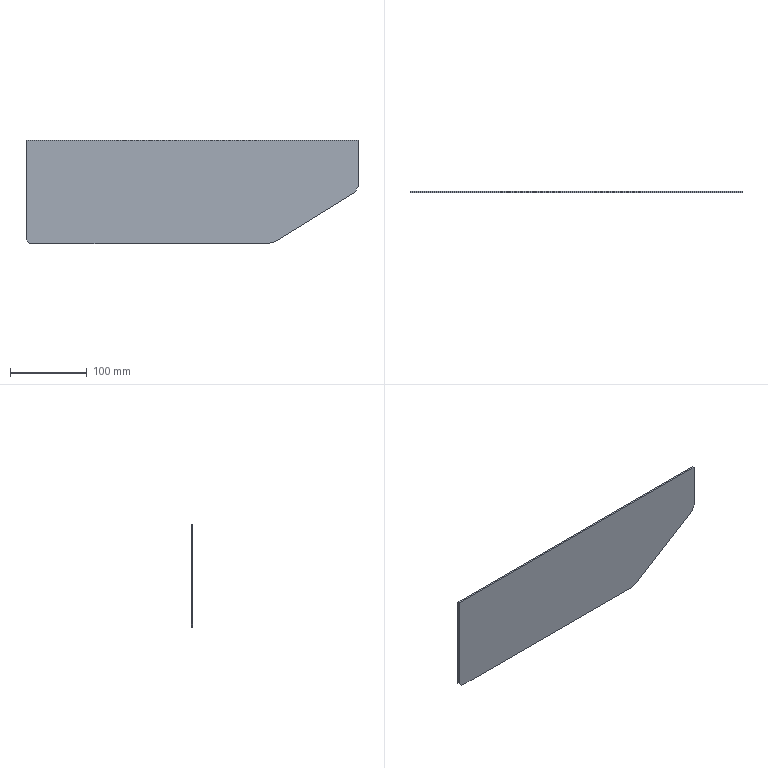Part | SolidWorks | features Chamfer 2, FlatPattern 1, SMBaseFlange 1, SheetMetal 1 | 1 solid | 10 faces | box 431.35 x 2.3 x 134 mm | volume 124034 mm3 | plane 10
STEP:
#1=CARTESIAN_POINT('',(0.,0.,-129.));
#2=VERTEX_POINT('',#1);
#3=CARTESIAN_POINT('',(0.,0.,0.));
#4=VERTEX_POINT('',#3);
#5=CARTESIAN_POINT('',(0.,0.,-134.));
#6=DIRECTION('',(0.,0.,1.));
#7=VECTOR('',#6,1000.);
#8=LINE('',#5,#7);
#9=EDGE_CURVE('',#2,#4,#8,.T.);
#10=ORIENTED_EDGE('',*,*,#9,.F.);
#11=CARTESIAN_POINT('',(0.,-2.3,-129.));
#12=VERTEX_POINT('',#11);
#13=CARTESIAN_POINT('',(0.,-2.3,-129.));
#14=DIRECTION('',(0.,-1.,0.));
#15=VECTOR('',#14,1000.);
#16=LINE('',#13,#15);
#17=EDGE_CURVE('',#2,#12,#16,.T.);
#18=ORIENTED_EDGE('',*,*,#17,.T.);
#19=CARTESIAN_POINT('',(0.,-2.3,0.));
#20=VERTEX_POINT('',#19);
#21=CARTESIAN_POINT('',(0.,-2.3,-134.));
#22=DIRECTION('',(0.,0.,1.));
#23=VECTOR('',#22,1000.);
#24=LINE('',#21,#23);
#25=EDGE_CURVE('',#12,#20,#24,.T.);
#26=ORIENTED_EDGE('',*,*,#25,.T.);
#27=CARTESIAN_POINT('',(0.,-2.3,0.));
#28=DIRECTION('',(0.,1.,0.));
#29=VECTOR('',#28,1000.);
#30=LINE('',#27,#29);
#31=EDGE_CURVE('',#20,#4,#30,.T.);
#32=ORIENTED_EDGE('',*,*,#31,.T.);
#33=EDGE_LOOP('',(#10,#18,#26,#32));
#34=FACE_OUTER_BOUND('',#33,.T.);
#35=CARTESIAN_POINT('',(0.,-2.3,-134.));
#36=DIRECTION('',(-1.,0.,0.));
#37=DIRECTION('',(0.,0.,1.));
#38=AXIS2_PLACEMENT_3D('',#35,#36,#37);
#39=PLANE('',#38);
#40=ADVANCED_FACE('',(#34),#39,.T.);
#41=CARTESIAN_POINT('',(314.95,-2.3,-134.));
#42=VERTEX_POINT('',#41);
#43=CARTESIAN_POINT('',(5.,-2.3,-134.));
#44=VERTEX_POINT('',#43);
#45=CARTESIAN_POINT('',(319.95,-2.3,-134.));
#46=DIRECTION('',(-1.,0.,0.));
#47=VECTOR('',#46,1000.);
#48=LINE('',#45,#47);
#49=EDGE_CURVE('',#42,#44,#48,.T.);
#50=ORIENTED_EDGE('',*,*,#49,.T.);
#51=CARTESIAN_POINT('',(5.,0.,-134.));
#52=VERTEX_POINT('',#51);
#53=CARTESIAN_POINT('',(5.,-2.3,-134.));
#54=DIRECTION('',(0.,1.,0.));
#55=VECTOR('',#54,1000.);
#56=LINE('',#53,#55);
#57=EDGE_CURVE('',#44,#52,#56,.T.);
#58=ORIENTED_EDGE('',*,*,#57,.T.);
#59=CARTESIAN_POINT('',(314.95,0.,-134.));
#60=VERTEX_POINT('',#59);
#61=CARTESIAN_POINT('',(319.95,0.,-134.));
#62=DIRECTION('',(-1.,0.,0.));
#63=VECTOR('',#62,1000.);
#64=LINE('',#61,#63);
#65=EDGE_CURVE('',#60,#52,#64,.T.);
#66=ORIENTED_EDGE('',*,*,#65,.F.);
#67=CARTESIAN_POINT('',(314.95,-2.3,-134.));
#68=DIRECTION('',(0.,-1.,0.));
#69=VECTOR('',#68,1000.);
#70=LINE('',#67,#69);
#71=EDGE_CURVE('',#60,#42,#70,.T.);
#72=ORIENTED_EDGE('',*,*,#71,.T.);
#73=EDGE_LOOP('',(#50,#58,#66,#72));
#74=FACE_OUTER_BOUND('',#73,.T.);
#75=CARTESIAN_POINT('',(319.95,-2.3,-134.));
#76=DIRECTION('',(0.,0.,-1.));
#77=DIRECTION('',(-1.,0.,0.));
#78=AXIS2_PLACEMENT_3D('',#75,#76,#77);
#79=PLANE('',#78);
#80=ADVANCED_FACE('',(#74),#79,.T.);
#81=CARTESIAN_POINT('',(427.099,0.,-67.633));
#82=VERTEX_POINT('',#81);
#83=CARTESIAN_POINT('',(324.201,0.,-131.367));
#84=VERTEX_POINT('',#83);
#85=CARTESIAN_POINT('',(431.35,0.,-65.));
#86=DIRECTION('',(-0.8501,0.,-0.5266));
#87=VECTOR('',#86,1000.);
#88=LINE('',#85,#87);
#89=EDGE_CURVE('',#82,#84,#88,.T.);
#90=ORIENTED_EDGE('',*,*,#89,.F.);
#91=CARTESIAN_POINT('',(427.099,-2.3,-67.633));
#92=VERTEX_POINT('',#91);
#93=CARTESIAN_POINT('',(427.099,-2.3,-67.633));
#94=DIRECTION('',(0.,-1.,0.));
#95=VECTOR('',#94,1000.);
#96=LINE('',#93,#95);
#97=EDGE_CURVE('',#82,#92,#96,.T.);
#98=ORIENTED_EDGE('',*,*,#97,.T.);
#99=CARTESIAN_POINT('',(324.201,-2.3,-131.367));
#100=VERTEX_POINT('',#99);
#101=CARTESIAN_POINT('',(431.35,-2.3,-65.));
#102=DIRECTION('',(-0.8501,0.,-0.5266));
#103=VECTOR('',#102,1000.);
#104=LINE('',#101,#103);
#105=EDGE_CURVE('',#92,#100,#104,.T.);
#106=ORIENTED_EDGE('',*,*,#105,.T.);
#107=CARTESIAN_POINT('',(324.201,-2.3,-131.367));
#108=DIRECTION('',(0.,1.,0.));
#109=VECTOR('',#108,1000.);
#110=LINE('',#107,#109);
#111=EDGE_CURVE('',#100,#84,#110,.T.);
#112=ORIENTED_EDGE('',*,*,#111,.T.);
#113=EDGE_LOOP('',(#90,#98,#106,#112));
#114=FACE_OUTER_BOUND('',#113,.T.);
#115=CARTESIAN_POINT('',(431.35,-2.3,-65.));
#116=DIRECTION('',(0.5266,0.,-0.8501));
#117=DIRECTION('',(-0.8501,0.,-0.5266));
#118=AXIS2_PLACEMENT_3D('',#115,#116,#117);
#119=PLANE('',#118);
#120=ADVANCED_FACE('',(#114),#119,.T.);
#121=CARTESIAN_POINT('',(431.35,-2.3,0.));
#122=VERTEX_POINT('',#121);
#123=CARTESIAN_POINT('',(431.35,-2.3,-60.));
#124=VERTEX_POINT('',#123);
#125=CARTESIAN_POINT('',(431.35,-2.3,0.));
#126=DIRECTION('',(0.,0.,-1.));
#127=VECTOR('',#126,1000.);
#128=LINE('',#125,#127);
#129=EDGE_CURVE('',#122,#124,#128,.T.);
#130=ORIENTED_EDGE('',*,*,#129,.T.);
#131=CARTESIAN_POINT('',(431.35,0.,-60.));
#132=VERTEX_POINT('',#131);
#133=CARTESIAN_POINT('',(431.35,-2.3,-60.));
#134=DIRECTION('',(0.,1.,0.));
#135=VECTOR('',#134,1000.);
#136=LINE('',#133,#135);
#137=EDGE_CURVE('',#124,#132,#136,.T.);
#138=ORIENTED_EDGE('',*,*,#137,.T.);
#139=CARTESIAN_POINT('',(431.35,0.,0.));
#140=VERTEX_POINT('',#139);
#141=CARTESIAN_POINT('',(431.35,0.,0.));
#142=DIRECTION('',(0.,0.,-1.));
#143=VECTOR('',#142,1000.);
#144=LINE('',#141,#143);
#145=EDGE_CURVE('',#140,#132,#144,.T.);
#146=ORIENTED_EDGE('',*,*,#145,.F.);
#147=CARTESIAN_POINT('',(431.35,-2.3,0.));
#148=DIRECTION('',(0.,1.,0.));
#149=VECTOR('',#148,1000.);
#150=LINE('',#147,#149);
#151=EDGE_CURVE('',#122,#140,#150,.T.);
#152=ORIENTED_EDGE('',*,*,#151,.F.);
#153=EDGE_LOOP('',(#130,#138,#146,#152));
#154=FACE_OUTER_BOUND('',#153,.T.);
#155=CARTESIAN_POINT('',(431.35,-2.3,0.));
#156=DIRECTION('',(1.,0.,0.));
#157=DIRECTION('',(0.,0.,-1.));
#158=AXIS2_PLACEMENT_3D('',#155,#156,#157);
#159=PLANE('',#158);
#160=ADVANCED_FACE('',(#154),#159,.T.);
#161=CARTESIAN_POINT('',(0.,0.,0.));
#162=DIRECTION('',(1.,0.,0.));
#163=VECTOR('',#162,1000.);
#164=LINE('',#161,#163);
#165=EDGE_CURVE('',#4,#140,#164,.T.);
#166=ORIENTED_EDGE('',*,*,#165,.F.);
#167=ORIENTED_EDGE('',*,*,#31,.F.);
#168=CARTESIAN_POINT('',(0.,-2.3,0.));
#169=DIRECTION('',(1.,0.,0.));
#170=VECTOR('',#169,1000.);
#171=LINE('',#168,#170);
#172=EDGE_CURVE('',#20,#122,#171,.T.);
#173=ORIENTED_EDGE('',*,*,#172,.T.);
#174=ORIENTED_EDGE('',*,*,#151,.T.);
#175=EDGE_LOOP('',(#166,#167,#173,#174));
#176=FACE_OUTER_BOUND('',#175,.T.);
#177=CARTESIAN_POINT('',(0.,-2.3,0.));
#178=DIRECTION('',(0.,0.,1.));
#179=DIRECTION('',(1.,0.,0.));
#180=AXIS2_PLACEMENT_3D('',#177,#178,#179);
#181=PLANE('',#180);
#182=ADVANCED_FACE('',(#176),#181,.T.);
#183=ORIENTED_EDGE('',*,*,#25,.F.);
#184=CARTESIAN_POINT('',(5.,-2.3,-134.));
#185=DIRECTION('',(0.7071,0.,-0.7071));
#186=VECTOR('',#185,1000.);
#187=LINE('',#184,#186);
#188=EDGE_CURVE('',#12,#44,#187,.T.);
#189=ORIENTED_EDGE('',*,*,#188,.T.);
#190=ORIENTED_EDGE('',*,*,#49,.F.);
#191=CARTESIAN_POINT('',(324.201,-2.3,-131.367));
#192=DIRECTION('',(0.9618,0.,0.2737));
#193=VECTOR('',#192,1000.);
#194=LINE('',#191,#193);
#195=EDGE_CURVE('',#42,#100,#194,.T.);
#196=ORIENTED_EDGE('',*,*,#195,.T.);
#197=ORIENTED_EDGE('',*,*,#105,.F.);
#198=CARTESIAN_POINT('',(431.35,-2.3,-60.));
#199=DIRECTION('',(0.4865,0.,0.8737));
#200=VECTOR('',#199,1000.);
#201=LINE('',#198,#200);
#202=EDGE_CURVE('',#92,#124,#201,.T.);
#203=ORIENTED_EDGE('',*,*,#202,.T.);
#204=ORIENTED_EDGE('',*,*,#129,.F.);
#205=ORIENTED_EDGE('',*,*,#172,.F.);
#206=EDGE_LOOP('',(#183,#189,#190,#196,#197,#203,#204,#205));
#207=FACE_OUTER_BOUND('',#206,.T.);
#208=CARTESIAN_POINT('',(0.,-2.3,0.));
#209=DIRECTION('',(0.,1.,0.));
#210=DIRECTION('',(0.,0.,1.));
#211=AXIS2_PLACEMENT_3D('',#208,#209,#210);
#212=PLANE('',#211);
#213=ADVANCED_FACE('',(#207),#212,.F.);
#214=ORIENTED_EDGE('',*,*,#65,.T.);
#215=CARTESIAN_POINT('',(-64.5,0.,-64.5));
#216=DIRECTION('',(-0.7071,0.,0.7071));
#217=VECTOR('',#216,1000.);
#218=LINE('',#215,#217);
#219=EDGE_CURVE('',#52,#2,#218,.T.);
#220=ORIENTED_EDGE('',*,*,#219,.T.);
#221=ORIENTED_EDGE('',*,*,#9,.T.);
#222=ORIENTED_EDGE('',*,*,#165,.T.);
#223=ORIENTED_EDGE('',*,*,#145,.T.);
#224=CARTESIAN_POINT('',(354.746,0.,-197.556));
#225=DIRECTION('',(-0.4865,0.,-0.8737));
#226=VECTOR('',#225,1000.);
#227=LINE('',#224,#226);
#228=EDGE_CURVE('',#132,#82,#227,.T.);
#229=ORIENTED_EDGE('',*,*,#228,.T.);
#230=ORIENTED_EDGE('',*,*,#89,.T.);
#231=CARTESIAN_POINT('',(58.88,0.,-206.88));
#232=DIRECTION('',(-0.9618,0.,-0.2737));
#233=VECTOR('',#232,1000.);
#234=LINE('',#231,#233);
#235=EDGE_CURVE('',#84,#60,#234,.T.);
#236=ORIENTED_EDGE('',*,*,#235,.T.);
#237=EDGE_LOOP('',(#214,#220,#221,#222,#223,#229,#230,#236));
#238=FACE_OUTER_BOUND('',#237,.T.);
#239=CARTESIAN_POINT('',(0.,0.,0.));
#240=DIRECTION('',(0.,1.,0.));
#241=DIRECTION('',(0.,0.,1.));
#242=AXIS2_PLACEMENT_3D('',#239,#240,#241);
#243=PLANE('',#242);
#244=ADVANCED_FACE('',(#238),#243,.T.);
#245=ORIENTED_EDGE('',*,*,#202,.F.);
#246=ORIENTED_EDGE('',*,*,#97,.F.);
#247=ORIENTED_EDGE('',*,*,#228,.F.);
#248=ORIENTED_EDGE('',*,*,#137,.F.);
#249=EDGE_LOOP('',(#245,#246,#247,#248));
#250=FACE_OUTER_BOUND('',#249,.T.);
#251=CARTESIAN_POINT('',(431.35,-2.3,-60.));
#252=DIRECTION('',(-0.8737,0.,0.4865));
#253=DIRECTION('',(0.,1.,0.));
#254=AXIS2_PLACEMENT_3D('',#251,#252,#253);
#255=PLANE('',#254);
#256=ADVANCED_FACE('',(#250),#255,.F.);
#257=ORIENTED_EDGE('',*,*,#195,.F.);
#258=ORIENTED_EDGE('',*,*,#71,.F.);
#259=ORIENTED_EDGE('',*,*,#235,.F.);
#260=ORIENTED_EDGE('',*,*,#111,.F.);
#261=EDGE_LOOP('',(#257,#258,#259,#260));
#262=FACE_OUTER_BOUND('',#261,.T.);
#263=CARTESIAN_POINT('',(324.201,-2.3,-131.367));
#264=DIRECTION('',(-0.2737,0.,0.9618));
#265=DIRECTION('',(0.,1.,0.));
#266=AXIS2_PLACEMENT_3D('',#263,#264,#265);
#267=PLANE('',#266);
#268=ADVANCED_FACE('',(#262),#267,.F.);
#269=ORIENTED_EDGE('',*,*,#188,.F.);
#270=ORIENTED_EDGE('',*,*,#17,.F.);
#271=ORIENTED_EDGE('',*,*,#219,.F.);
#272=ORIENTED_EDGE('',*,*,#57,.F.);
#273=EDGE_LOOP('',(#269,#270,#271,#272));
#274=FACE_OUTER_BOUND('',#273,.T.);
#275=CARTESIAN_POINT('',(5.,-2.3,-134.));
#276=DIRECTION('',(0.7071,0.,0.7071));
#277=DIRECTION('',(0.,1.,0.));
#278=AXIS2_PLACEMENT_3D('',#275,#276,#277);
#279=PLANE('',#278);
#280=ADVANCED_FACE('',(#274),#279,.F.);
#281=CLOSED_SHELL('',(#40,#80,#120,#160,#182,#213,#244,#256,#268,#280));
#282=MANIFOLD_SOLID_BREP('',#281);
#283=CARTESIAN_POINT('',(0.,0.,0.));
#284=DIRECTION('',(0.,0.,1.));
#285=DIRECTION('',(1.,0.,0.));
#286=AXIS2_PLACEMENT_3D('',#283,#284,#285);
#287=(LENGTH_UNIT()NAMED_UNIT(*)SI_UNIT(.MILLI.,.METRE.));
#288=UNCERTAINTY_MEASURE_WITH_UNIT(LENGTH_MEASURE(0.00001),#287,'','');
#289=(NAMED_UNIT(*)PLANE_ANGLE_UNIT()SI_UNIT($,.RADIAN.));
#290=(NAMED_UNIT(*)SI_UNIT($,.STERADIAN.)SOLID_ANGLE_UNIT());
#291=(GEOMETRIC_REPRESENTATION_CONTEXT(3)GLOBAL_UNCERTAINTY_ASSIGNED_CONTEXT((#288))GLOBAL_UNIT_ASSIGNED_CONTEXT((#287,#289,#290))REPRESENTATION_CONTEXT('',''));
#292=ADVANCED_BREP_SHAPE_REPRESENTATION('',(#282,#286),#291);